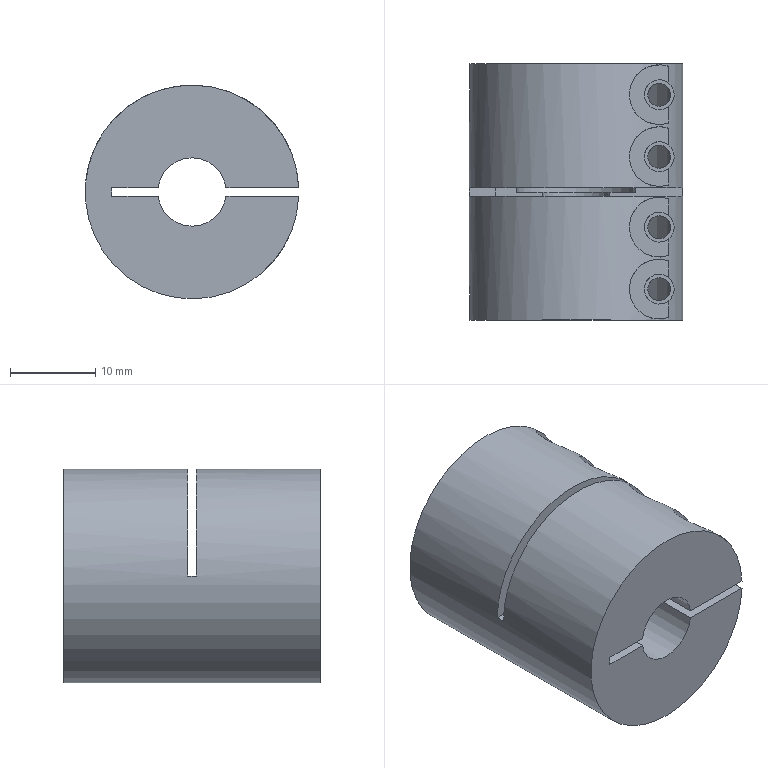Part | NX | features SIMPLE HOLE 14, DATUM_CSYS 6, SYMBOLIC_THREAD 6, SKETCH 5, EXTRUDE 4, HOLE PACKAGE 3, ASSOCIATIVE_INTERSECTION 1, SWP104 1 | 1 solid | 42 faces | box 24.99 x 30 x 25 mm | volume 10501 mm3 | cylinder 21 | plane 17 | spline 4 | commonest cylinder face diameters 25 x5 2.7 x4 3.5 x4 7 x4 8 x2 14 x2